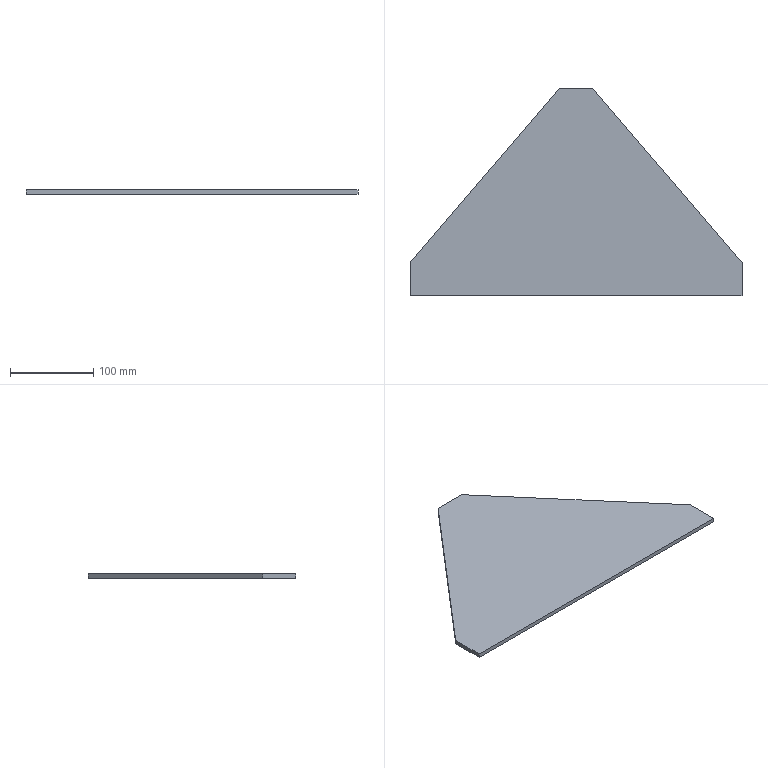Part | SolidWorks | features Extrusion 1, ICE 1 | 1 solid | 8 faces | box 400 x 250 x 5 mm | volume 311000 mm3 | plane 8
STEP:
#1=CARTESIAN_POINT('',(-200.,-85.,0.));
#2=VERTEX_POINT('',#1);
#3=CARTESIAN_POINT('',(-200.,-85.,5.));
#4=VERTEX_POINT('',#3);
#5=CARTESIAN_POINT('',(-200.,-85.,0.));
#6=DIRECTION('',(0.,0.,1.));
#7=VECTOR('',#6,1000.);
#8=LINE('',#5,#7);
#9=EDGE_CURVE('',#2,#4,#8,.T.);
#10=ORIENTED_EDGE('',*,*,#9,.F.);
#11=CARTESIAN_POINT('',(-200.,-125.,0.));
#12=VERTEX_POINT('',#11);
#13=CARTESIAN_POINT('',(-200.,125.,0.));
#14=DIRECTION('',(0.,-1.,0.));
#15=VECTOR('',#14,1000.);
#16=LINE('',#13,#15);
#17=EDGE_CURVE('',#2,#12,#16,.T.);
#18=ORIENTED_EDGE('',*,*,#17,.T.);
#19=CARTESIAN_POINT('',(-200.,-125.,5.));
#20=VERTEX_POINT('',#19);
#21=CARTESIAN_POINT('',(-200.,-125.,5.));
#22=DIRECTION('',(0.,0.,-1.));
#23=VECTOR('',#22,1000.);
#24=LINE('',#21,#23);
#25=EDGE_CURVE('',#20,#12,#24,.T.);
#26=ORIENTED_EDGE('',*,*,#25,.F.);
#27=CARTESIAN_POINT('',(-200.,125.,5.));
#28=DIRECTION('',(0.,-1.,0.));
#29=VECTOR('',#28,1000.);
#30=LINE('',#27,#29);
#31=EDGE_CURVE('',#4,#20,#30,.T.);
#32=ORIENTED_EDGE('',*,*,#31,.F.);
#33=EDGE_LOOP('',(#10,#18,#26,#32));
#34=FACE_OUTER_BOUND('',#33,.T.);
#35=CARTESIAN_POINT('',(-200.,125.,5.));
#36=DIRECTION('',(1.,0.,0.));
#37=DIRECTION('',(0.,1.,0.));
#38=AXIS2_PLACEMENT_3D('',#35,#36,#37);
#39=PLANE('',#38);
#40=ADVANCED_FACE('',(#34),#39,.F.);
#41=CARTESIAN_POINT('',(200.,-85.,0.));
#42=VERTEX_POINT('',#41);
#43=CARTESIAN_POINT('',(200.,-85.,5.));
#44=VERTEX_POINT('',#43);
#45=CARTESIAN_POINT('',(200.,-85.,0.));
#46=DIRECTION('',(0.,0.,1.));
#47=VECTOR('',#46,1000.);
#48=LINE('',#45,#47);
#49=EDGE_CURVE('',#42,#44,#48,.T.);
#50=ORIENTED_EDGE('',*,*,#49,.T.);
#51=CARTESIAN_POINT('',(200.,-125.,5.));
#52=VERTEX_POINT('',#51);
#53=CARTESIAN_POINT('',(200.,125.,5.));
#54=DIRECTION('',(0.,1.,0.));
#55=VECTOR('',#54,1000.);
#56=LINE('',#53,#55);
#57=EDGE_CURVE('',#52,#44,#56,.T.);
#58=ORIENTED_EDGE('',*,*,#57,.F.);
#59=CARTESIAN_POINT('',(200.,-125.,0.));
#60=VERTEX_POINT('',#59);
#61=CARTESIAN_POINT('',(200.,-125.,5.));
#62=DIRECTION('',(0.,0.,-1.));
#63=VECTOR('',#62,1000.);
#64=LINE('',#61,#63);
#65=EDGE_CURVE('',#52,#60,#64,.T.);
#66=ORIENTED_EDGE('',*,*,#65,.T.);
#67=CARTESIAN_POINT('',(200.,125.,0.));
#68=DIRECTION('',(0.,1.,0.));
#69=VECTOR('',#68,1000.);
#70=LINE('',#67,#69);
#71=EDGE_CURVE('',#60,#42,#70,.T.);
#72=ORIENTED_EDGE('',*,*,#71,.T.);
#73=EDGE_LOOP('',(#50,#58,#66,#72));
#74=FACE_OUTER_BOUND('',#73,.T.);
#75=CARTESIAN_POINT('',(200.,125.,5.));
#76=DIRECTION('',(-1.,0.,0.));
#77=DIRECTION('',(0.,-1.,0.));
#78=AXIS2_PLACEMENT_3D('',#75,#76,#77);
#79=PLANE('',#78);
#80=ADVANCED_FACE('',(#74),#79,.F.);
#81=CARTESIAN_POINT('',(-20.,125.,0.));
#82=VERTEX_POINT('',#81);
#83=CARTESIAN_POINT('',(-20.,125.,5.));
#84=VERTEX_POINT('',#83);
#85=CARTESIAN_POINT('',(-20.,125.,0.));
#86=DIRECTION('',(0.,0.,1.));
#87=VECTOR('',#86,1000.);
#88=LINE('',#85,#87);
#89=EDGE_CURVE('',#82,#84,#88,.T.);
#90=ORIENTED_EDGE('',*,*,#89,.T.);
#91=CARTESIAN_POINT('',(20.,125.,5.));
#92=VERTEX_POINT('',#91);
#93=CARTESIAN_POINT('',(200.,125.,5.));
#94=DIRECTION('',(-1.,0.,0.));
#95=VECTOR('',#94,1000.);
#96=LINE('',#93,#95);
#97=EDGE_CURVE('',#92,#84,#96,.T.);
#98=ORIENTED_EDGE('',*,*,#97,.F.);
#99=CARTESIAN_POINT('',(20.,125.,0.));
#100=VERTEX_POINT('',#99);
#101=CARTESIAN_POINT('',(20.,125.,0.));
#102=DIRECTION('',(0.,0.,1.));
#103=VECTOR('',#102,1000.);
#104=LINE('',#101,#103);
#105=EDGE_CURVE('',#100,#92,#104,.T.);
#106=ORIENTED_EDGE('',*,*,#105,.F.);
#107=CARTESIAN_POINT('',(200.,125.,0.));
#108=DIRECTION('',(-1.,0.,0.));
#109=VECTOR('',#108,1000.);
#110=LINE('',#107,#109);
#111=EDGE_CURVE('',#100,#82,#110,.T.);
#112=ORIENTED_EDGE('',*,*,#111,.T.);
#113=EDGE_LOOP('',(#90,#98,#106,#112));
#114=FACE_OUTER_BOUND('',#113,.T.);
#115=CARTESIAN_POINT('',(200.,125.,5.));
#116=DIRECTION('',(0.,-1.,0.));
#117=DIRECTION('',(1.,0.,0.));
#118=AXIS2_PLACEMENT_3D('',#115,#116,#117);
#119=PLANE('',#118);
#120=ADVANCED_FACE('',(#114),#119,.F.);
#121=CARTESIAN_POINT('',(-200.,-85.,5.));
#122=DIRECTION('',(-0.6508,-0.7593,0.));
#123=VECTOR('',#122,1000.);
#124=LINE('',#121,#123);
#125=EDGE_CURVE('',#84,#4,#124,.T.);
#126=ORIENTED_EDGE('',*,*,#125,.T.);
#127=ORIENTED_EDGE('',*,*,#31,.T.);
#128=CARTESIAN_POINT('',(200.,-125.,5.));
#129=DIRECTION('',(1.,0.,0.));
#130=VECTOR('',#129,1000.);
#131=LINE('',#128,#130);
#132=EDGE_CURVE('',#20,#52,#131,.T.);
#133=ORIENTED_EDGE('',*,*,#132,.T.);
#134=ORIENTED_EDGE('',*,*,#57,.T.);
#135=CARTESIAN_POINT('',(20.,125.,5.));
#136=DIRECTION('',(-0.6508,0.7593,0.));
#137=VECTOR('',#136,1000.);
#138=LINE('',#135,#137);
#139=EDGE_CURVE('',#44,#92,#138,.T.);
#140=ORIENTED_EDGE('',*,*,#139,.T.);
#141=ORIENTED_EDGE('',*,*,#97,.T.);
#142=EDGE_LOOP('',(#126,#127,#133,#134,#140,#141));
#143=FACE_OUTER_BOUND('',#142,.T.);
#144=CARTESIAN_POINT('',(0.,0.,5.));
#145=DIRECTION('',(0.,0.,-1.));
#146=DIRECTION('',(-1.,0.,0.));
#147=AXIS2_PLACEMENT_3D('',#144,#145,#146);
#148=PLANE('',#147);
#149=ADVANCED_FACE('',(#143),#148,.F.);
#150=ORIENTED_EDGE('',*,*,#17,.F.);
#151=CARTESIAN_POINT('',(-200.,-85.,0.));
#152=DIRECTION('',(-0.6508,-0.7593,0.));
#153=VECTOR('',#152,1000.);
#154=LINE('',#151,#153);
#155=EDGE_CURVE('',#82,#2,#154,.T.);
#156=ORIENTED_EDGE('',*,*,#155,.F.);
#157=ORIENTED_EDGE('',*,*,#111,.F.);
#158=CARTESIAN_POINT('',(20.,125.,0.));
#159=DIRECTION('',(-0.6508,0.7593,0.));
#160=VECTOR('',#159,1000.);
#161=LINE('',#158,#160);
#162=EDGE_CURVE('',#42,#100,#161,.T.);
#163=ORIENTED_EDGE('',*,*,#162,.F.);
#164=ORIENTED_EDGE('',*,*,#71,.F.);
#165=CARTESIAN_POINT('',(200.,-125.,0.));
#166=DIRECTION('',(1.,0.,0.));
#167=VECTOR('',#166,1000.);
#168=LINE('',#165,#167);
#169=EDGE_CURVE('',#12,#60,#168,.T.);
#170=ORIENTED_EDGE('',*,*,#169,.F.);
#171=EDGE_LOOP('',(#150,#156,#157,#163,#164,#170));
#172=FACE_OUTER_BOUND('',#171,.T.);
#173=CARTESIAN_POINT('',(0.,0.,0.));
#174=DIRECTION('',(0.,0.,-1.));
#175=DIRECTION('',(-1.,0.,0.));
#176=AXIS2_PLACEMENT_3D('',#173,#174,#175);
#177=PLANE('',#176);
#178=ADVANCED_FACE('',(#172),#177,.T.);
#179=ORIENTED_EDGE('',*,*,#169,.T.);
#180=ORIENTED_EDGE('',*,*,#65,.F.);
#181=ORIENTED_EDGE('',*,*,#132,.F.);
#182=ORIENTED_EDGE('',*,*,#25,.T.);
#183=EDGE_LOOP('',(#179,#180,#181,#182));
#184=FACE_OUTER_BOUND('',#183,.T.);
#185=CARTESIAN_POINT('',(200.,-125.,5.));
#186=DIRECTION('',(0.,1.,0.));
#187=DIRECTION('',(-1.,0.,0.));
#188=AXIS2_PLACEMENT_3D('',#185,#186,#187);
#189=PLANE('',#188);
#190=ADVANCED_FACE('',(#184),#189,.F.);
#191=ORIENTED_EDGE('',*,*,#139,.F.);
#192=ORIENTED_EDGE('',*,*,#49,.F.);
#193=ORIENTED_EDGE('',*,*,#162,.T.);
#194=ORIENTED_EDGE('',*,*,#105,.T.);
#195=EDGE_LOOP('',(#191,#192,#193,#194));
#196=FACE_OUTER_BOUND('',#195,.T.);
#197=CARTESIAN_POINT('',(20.,125.,0.));
#198=DIRECTION('',(0.7593,0.6508,0.));
#199=DIRECTION('',(-0.6508,0.7593,0.));
#200=AXIS2_PLACEMENT_3D('',#197,#198,#199);
#201=PLANE('',#200);
#202=ADVANCED_FACE('',(#196),#201,.T.);
#203=ORIENTED_EDGE('',*,*,#125,.F.);
#204=ORIENTED_EDGE('',*,*,#89,.F.);
#205=ORIENTED_EDGE('',*,*,#155,.T.);
#206=ORIENTED_EDGE('',*,*,#9,.T.);
#207=EDGE_LOOP('',(#203,#204,#205,#206));
#208=FACE_OUTER_BOUND('',#207,.T.);
#209=CARTESIAN_POINT('',(-200.,-85.,0.));
#210=DIRECTION('',(-0.7593,0.6508,0.));
#211=DIRECTION('',(-0.6508,-0.7593,0.));
#212=AXIS2_PLACEMENT_3D('',#209,#210,#211);
#213=PLANE('',#212);
#214=ADVANCED_FACE('',(#208),#213,.T.);
#215=CLOSED_SHELL('',(#40,#80,#120,#149,#178,#190,#202,#214));
#216=MANIFOLD_SOLID_BREP('',#215);
#217=CARTESIAN_POINT('',(0.,0.,0.));
#218=DIRECTION('',(0.,0.,1.));
#219=DIRECTION('',(1.,0.,0.));
#220=AXIS2_PLACEMENT_3D('',#217,#218,#219);
#221=(LENGTH_UNIT()NAMED_UNIT(*)SI_UNIT(.MILLI.,.METRE.));
#222=UNCERTAINTY_MEASURE_WITH_UNIT(LENGTH_MEASURE(0.00001),#221,'','');
#223=(NAMED_UNIT(*)PLANE_ANGLE_UNIT()SI_UNIT($,.RADIAN.));
#224=(NAMED_UNIT(*)SI_UNIT($,.STERADIAN.)SOLID_ANGLE_UNIT());
#225=(GEOMETRIC_REPRESENTATION_CONTEXT(3)GLOBAL_UNCERTAINTY_ASSIGNED_CONTEXT((#222))GLOBAL_UNIT_ASSIGNED_CONTEXT((#221,#223,#224))REPRESENTATION_CONTEXT('',''));
#226=ADVANCED_BREP_SHAPE_REPRESENTATION('',(#216,#220),#225);